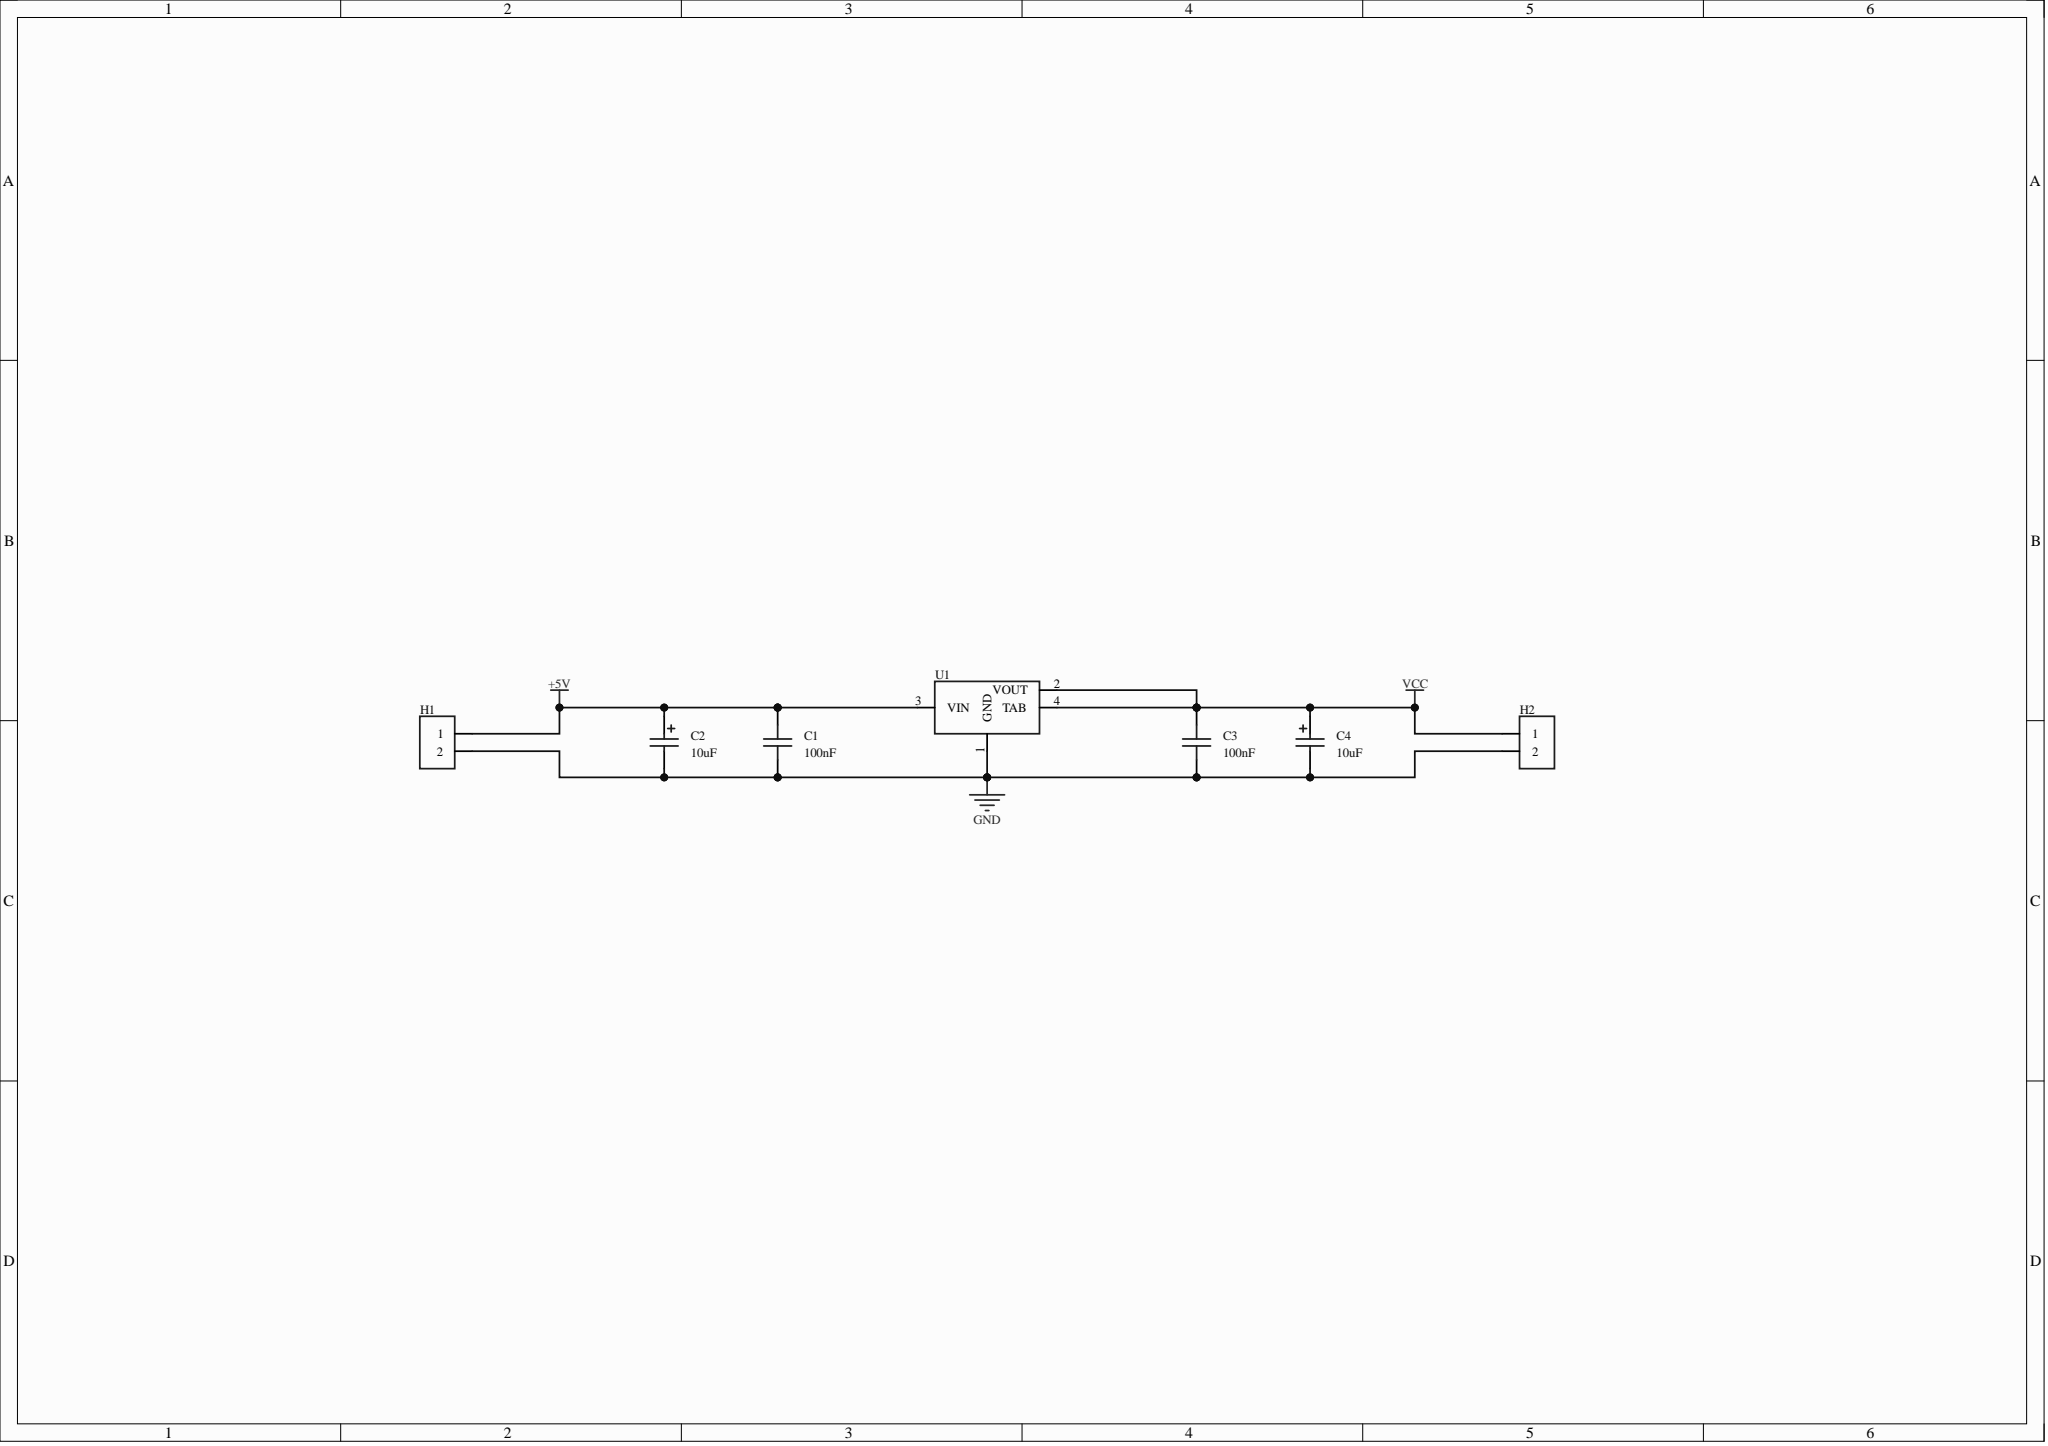Circuit board | Altium Designer | 7 parts | 3 nets
Bill of materials:
Comment,Description,Designator,Footprint,LibRef,Quantity
"100nF","","C1, C3","C0603","CAP_0603","2"
"10uF","","C2, C4","C_Ele_SMD_3x5.4mm","C_Ele_SMD_3x5.4mm","2"
"","","H1, H2","HDR-TH_2P-P2.54-V-F","HDR-F_2.54_1x2P","2"
"","","U1","SOT_223","AMS1117","1"
Netlist (Protel format):
[
C1
C0603
100nF



]
[
C2
C_Ele_SMD_3x5.4mm
10uF



]
[
C3
C0603
100nF



]
[
C4
C_Ele_SMD_3x5.4mm
10uF



]
[
H1
HDR-TH_2P-P2.54-V-F




]
[
H2
HDR-TH_2P-P2.54-V-F




]
[
U1
SOT_223




]
(
VCC
C3-2
C4-1
H2-1
U1-2
U1-4
)
(
GND
C1-1
C2-2
C3-1
C4-2
H1-2
H2-2
U1-1
)
(
+5V
C1-2
C2-1
H1-1
U1-3
)